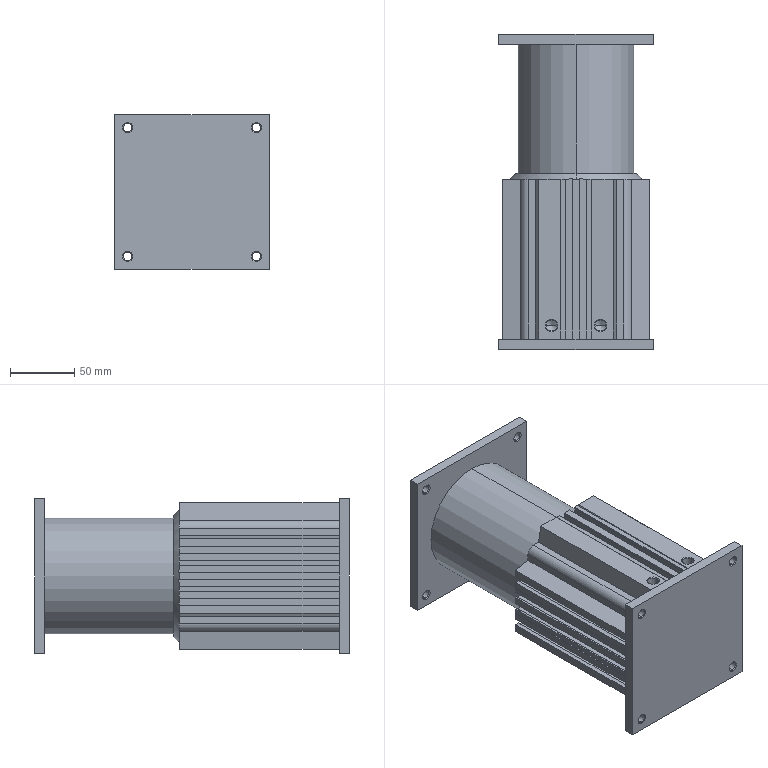Part | SolidWorks | features AEMSimFeature 1 | 2 solids | 301 faces | box 120 x 244.5 x 120 mm | volume 1424542 mm3 | plane 223 | cone 42 | cylinder 36 | commonest cylinder face diameters 6.647 x16 8.566 x4 12 x4 20 x4 40 x4 90 x4